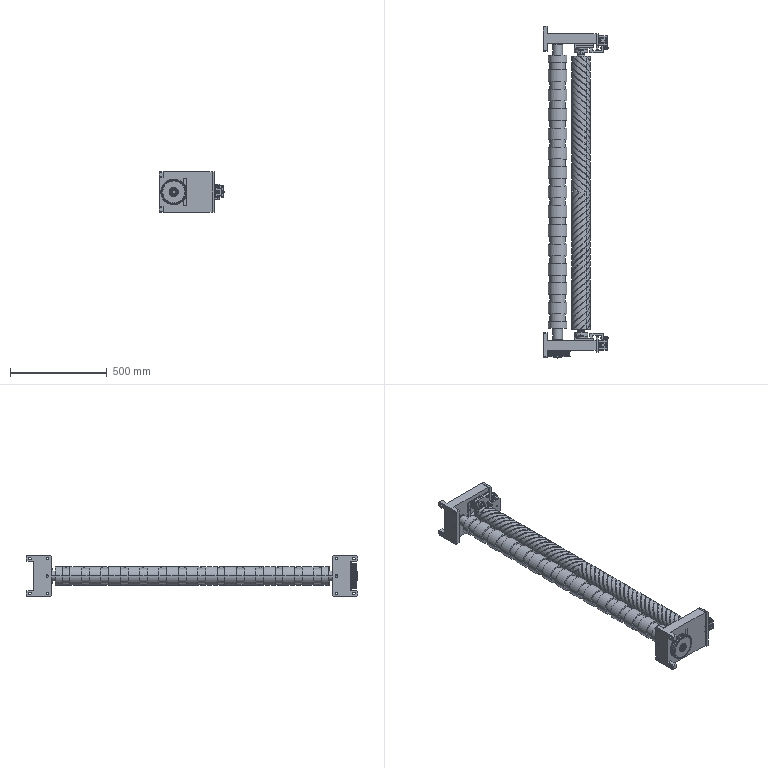Part | SolidWorks | 54 solids | 3493 faces | volume 25836003 mm3 | cylinder 1613 | plane 1176 | cone 386 | spline 126 | torus 124 | sphere 68 | commonest cylinder face diameters 0.5 x198 96 x130 3.143 x117 0.4 x92 126.211 x80 5.2 x72